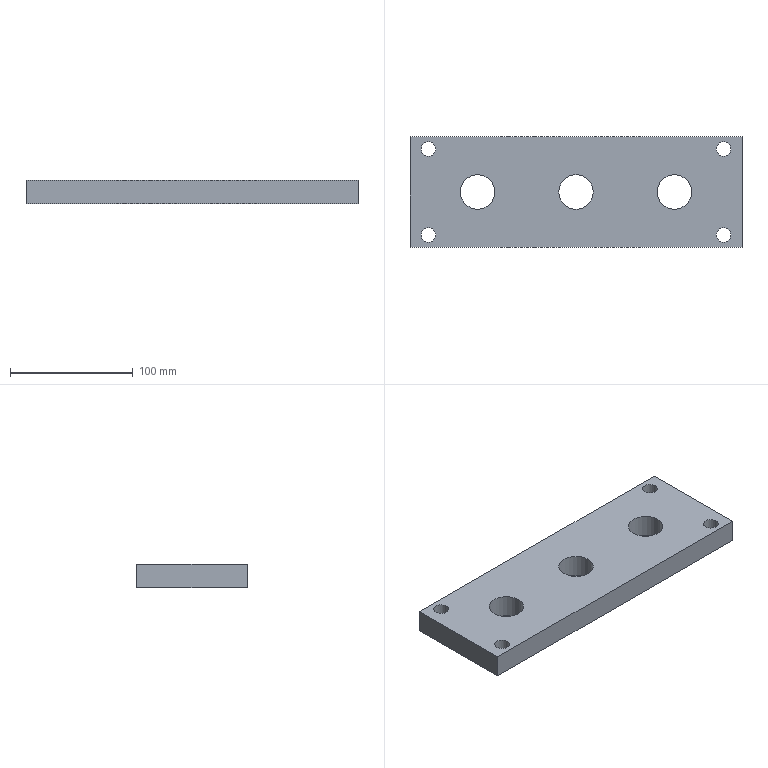Part | NX | features solid 2 | 1 solid | 13 faces | box 270 x 90 x 19 mm | volume 418007 mm3 | cylinder 7 | plane 6 | commonest cylinder face diameters 12 x4 28 x3
STEP:
#1=CARTESIAN_POINT('',(135.,-105.,-30.));
#2=VERTEX_POINT('',#1);
#3=CARTESIAN_POINT('',(-135.,-105.,-30.));
#4=VERTEX_POINT('',#3);
#5=CARTESIAN_POINT('',(165.,-105.,-30.));
#6=DIRECTION('',(-1.,0.,0.));
#7=VECTOR('',#6,1000.);
#8=LINE('',#5,#7);
#9=EDGE_CURVE('',#2,#4,#8,.T.);
#10=ORIENTED_EDGE('',*,*,#9,.T.);
#11=CARTESIAN_POINT('',(-135.,-105.,-49.));
#12=VERTEX_POINT('',#11);
#13=CARTESIAN_POINT('',(-135.,-105.,-30.));
#14=DIRECTION('',(0.,0.,-1.));
#15=VECTOR('',#14,1000.);
#16=LINE('',#13,#15);
#17=EDGE_CURVE('',#4,#12,#16,.T.);
#18=ORIENTED_EDGE('',*,*,#17,.T.);
#19=CARTESIAN_POINT('',(135.,-105.,-49.));
#20=VERTEX_POINT('',#19);
#21=CARTESIAN_POINT('',(-165.,-105.,-49.));
#22=DIRECTION('',(1.,0.,0.));
#23=VECTOR('',#22,1000.);
#24=LINE('',#21,#23);
#25=EDGE_CURVE('',#12,#20,#24,.T.);
#26=ORIENTED_EDGE('',*,*,#25,.T.);
#27=CARTESIAN_POINT('',(135.,-105.,-30.));
#28=DIRECTION('',(0.,0.,-1.));
#29=VECTOR('',#28,1000.);
#30=LINE('',#27,#29);
#31=EDGE_CURVE('',#2,#20,#30,.T.);
#32=ORIENTED_EDGE('',*,*,#31,.F.);
#33=EDGE_LOOP('',(#10,#18,#26,#32));
#34=FACE_BOUND('',#33,.T.);
#35=CARTESIAN_POINT('',(-165.,-105.,-30.));
#36=DIRECTION('',(0.,1.,0.));
#37=DIRECTION('',(0.,0.,1.));
#38=AXIS2_PLACEMENT_3D('',#35,#36,#37);
#39=PLANE('',#38);
#40=ADVANCED_FACE('',(#34),#39,.F.);
#41=CARTESIAN_POINT('',(135.,-15.,-49.));
#42=VERTEX_POINT('',#41);
#43=CARTESIAN_POINT('',(-135.,-15.,-49.));
#44=VERTEX_POINT('',#43);
#45=CARTESIAN_POINT('',(165.,-15.,-49.));
#46=DIRECTION('',(-1.,0.,0.));
#47=VECTOR('',#46,1000.);
#48=LINE('',#45,#47);
#49=EDGE_CURVE('',#42,#44,#48,.T.);
#50=ORIENTED_EDGE('',*,*,#49,.T.);
#51=CARTESIAN_POINT('',(-135.,-15.,-30.));
#52=VERTEX_POINT('',#51);
#53=CARTESIAN_POINT('',(-135.,-15.,-30.));
#54=DIRECTION('',(0.,0.,-1.));
#55=VECTOR('',#54,1000.);
#56=LINE('',#53,#55);
#57=EDGE_CURVE('',#52,#44,#56,.T.);
#58=ORIENTED_EDGE('',*,*,#57,.F.);
#59=CARTESIAN_POINT('',(135.,-15.,-30.));
#60=VERTEX_POINT('',#59);
#61=CARTESIAN_POINT('',(-165.,-15.,-30.));
#62=DIRECTION('',(1.,0.,0.));
#63=VECTOR('',#62,1000.);
#64=LINE('',#61,#63);
#65=EDGE_CURVE('',#52,#60,#64,.T.);
#66=ORIENTED_EDGE('',*,*,#65,.T.);
#67=CARTESIAN_POINT('',(135.,-15.,-30.));
#68=DIRECTION('',(0.,0.,-1.));
#69=VECTOR('',#68,1000.);
#70=LINE('',#67,#69);
#71=EDGE_CURVE('',#60,#42,#70,.T.);
#72=ORIENTED_EDGE('',*,*,#71,.T.);
#73=EDGE_LOOP('',(#50,#58,#66,#72));
#74=FACE_BOUND('',#73,.T.);
#75=CARTESIAN_POINT('',(165.,-15.,-30.));
#76=DIRECTION('',(0.,-1.,0.));
#77=DIRECTION('',(1.,0.,0.));
#78=AXIS2_PLACEMENT_3D('',#75,#76,#77);
#79=PLANE('',#78);
#80=ADVANCED_FACE('',(#74),#79,.F.);
#81=CARTESIAN_POINT('',(-114.,-25.,-30.));
#82=VERTEX_POINT('',#81);
#83=CARTESIAN_POINT('',(-120.,-25.,-30.));
#84=DIRECTION('',(0.,0.,1.));
#85=DIRECTION('',(1.,0.,0.));
#86=AXIS2_PLACEMENT_3D('',#83,#84,#85);
#87=CIRCLE('',#86,6.);
#88=EDGE_CURVE('',#82,#82,#87,.T.);
#89=ORIENTED_EDGE('',*,*,#88,.T.);
#90=EDGE_LOOP('',(#89));
#91=FACE_BOUND('',#90,.T.);
#92=CARTESIAN_POINT('',(-114.,-25.,-49.));
#93=VERTEX_POINT('',#92);
#94=CARTESIAN_POINT('',(-120.,-25.,-49.));
#95=DIRECTION('',(0.,0.,1.));
#96=DIRECTION('',(1.,0.,0.));
#97=AXIS2_PLACEMENT_3D('',#94,#95,#96);
#98=CIRCLE('',#97,6.);
#99=EDGE_CURVE('',#93,#93,#98,.T.);
#100=ORIENTED_EDGE('',*,*,#99,.F.);
#101=EDGE_LOOP('',(#100));
#102=FACE_BOUND('',#101,.T.);
#103=CARTESIAN_POINT('',(-120.,-25.,-30.));
#104=DIRECTION('',(0.,0.,-1.));
#105=DIRECTION('',(-1.,0.,0.));
#106=AXIS2_PLACEMENT_3D('',#103,#104,#105);
#107=CYLINDRICAL_SURFACE('',#106,6.);
#108=ADVANCED_FACE('',(#91,#102),#107,.F.);
#109=CARTESIAN_POINT('',(-114.,-95.,-30.));
#110=VERTEX_POINT('',#109);
#111=CARTESIAN_POINT('',(-120.,-95.,-30.));
#112=DIRECTION('',(0.,0.,-1.));
#113=DIRECTION('',(1.,0.,0.));
#114=AXIS2_PLACEMENT_3D('',#111,#112,#113);
#115=CIRCLE('',#114,6.);
#116=EDGE_CURVE('',#110,#110,#115,.T.);
#117=ORIENTED_EDGE('',*,*,#116,.F.);
#118=EDGE_LOOP('',(#117));
#119=FACE_BOUND('',#118,.T.);
#120=CARTESIAN_POINT('',(-114.,-95.,-49.));
#121=VERTEX_POINT('',#120);
#122=CARTESIAN_POINT('',(-120.,-95.,-49.));
#123=DIRECTION('',(0.,0.,-1.));
#124=DIRECTION('',(1.,0.,0.));
#125=AXIS2_PLACEMENT_3D('',#122,#123,#124);
#126=CIRCLE('',#125,6.);
#127=EDGE_CURVE('',#121,#121,#126,.T.);
#128=ORIENTED_EDGE('',*,*,#127,.T.);
#129=EDGE_LOOP('',(#128));
#130=FACE_BOUND('',#129,.T.);
#131=CARTESIAN_POINT('',(-120.,-95.,-30.));
#132=DIRECTION('',(0.,0.,-1.));
#133=DIRECTION('',(-1.,0.,0.));
#134=AXIS2_PLACEMENT_3D('',#131,#132,#133);
#135=CYLINDRICAL_SURFACE('',#134,6.);
#136=ADVANCED_FACE('',(#119,#130),#135,.F.);
#137=CARTESIAN_POINT('',(114.,-25.,-30.));
#138=VERTEX_POINT('',#137);
#139=CARTESIAN_POINT('',(120.,-25.,-30.));
#140=DIRECTION('',(0.,0.,-1.));
#141=DIRECTION('',(-1.,0.,0.));
#142=AXIS2_PLACEMENT_3D('',#139,#140,#141);
#143=CIRCLE('',#142,6.);
#144=EDGE_CURVE('',#138,#138,#143,.T.);
#145=ORIENTED_EDGE('',*,*,#144,.F.);
#146=EDGE_LOOP('',(#145));
#147=FACE_BOUND('',#146,.T.);
#148=CARTESIAN_POINT('',(114.,-25.,-49.));
#149=VERTEX_POINT('',#148);
#150=CARTESIAN_POINT('',(120.,-25.,-49.));
#151=DIRECTION('',(0.,0.,-1.));
#152=DIRECTION('',(-1.,0.,0.));
#153=AXIS2_PLACEMENT_3D('',#150,#151,#152);
#154=CIRCLE('',#153,6.);
#155=EDGE_CURVE('',#149,#149,#154,.T.);
#156=ORIENTED_EDGE('',*,*,#155,.T.);
#157=EDGE_LOOP('',(#156));
#158=FACE_BOUND('',#157,.T.);
#159=CARTESIAN_POINT('',(120.,-25.,-30.));
#160=DIRECTION('',(0.,0.,-1.));
#161=DIRECTION('',(-1.,0.,0.));
#162=AXIS2_PLACEMENT_3D('',#159,#160,#161);
#163=CYLINDRICAL_SURFACE('',#162,6.);
#164=ADVANCED_FACE('',(#147,#158),#163,.F.);
#165=CARTESIAN_POINT('',(114.,-95.,-30.));
#166=VERTEX_POINT('',#165);
#167=CARTESIAN_POINT('',(120.,-95.,-30.));
#168=DIRECTION('',(0.,0.,1.));
#169=DIRECTION('',(-1.,0.,0.));
#170=AXIS2_PLACEMENT_3D('',#167,#168,#169);
#171=CIRCLE('',#170,6.);
#172=EDGE_CURVE('',#166,#166,#171,.T.);
#173=ORIENTED_EDGE('',*,*,#172,.T.);
#174=EDGE_LOOP('',(#173));
#175=FACE_BOUND('',#174,.T.);
#176=CARTESIAN_POINT('',(114.,-95.,-49.));
#177=VERTEX_POINT('',#176);
#178=CARTESIAN_POINT('',(120.,-95.,-49.));
#179=DIRECTION('',(0.,0.,1.));
#180=DIRECTION('',(-1.,0.,0.));
#181=AXIS2_PLACEMENT_3D('',#178,#179,#180);
#182=CIRCLE('',#181,6.);
#183=EDGE_CURVE('',#177,#177,#182,.T.);
#184=ORIENTED_EDGE('',*,*,#183,.F.);
#185=EDGE_LOOP('',(#184));
#186=FACE_BOUND('',#185,.T.);
#187=CARTESIAN_POINT('',(120.,-95.,-30.));
#188=DIRECTION('',(0.,0.,-1.));
#189=DIRECTION('',(-1.,0.,0.));
#190=AXIS2_PLACEMENT_3D('',#187,#188,#189);
#191=CYLINDRICAL_SURFACE('',#190,6.);
#192=ADVANCED_FACE('',(#175,#186),#191,.F.);
#193=CARTESIAN_POINT('',(66.,-60.,-30.));
#194=VERTEX_POINT('',#193);
#195=CARTESIAN_POINT('',(80.,-60.,-30.));
#196=DIRECTION('',(0.,0.,-1.));
#197=DIRECTION('',(-1.,0.,0.));
#198=AXIS2_PLACEMENT_3D('',#195,#196,#197);
#199=CIRCLE('',#198,14.);
#200=EDGE_CURVE('',#194,#194,#199,.T.);
#201=ORIENTED_EDGE('',*,*,#200,.F.);
#202=EDGE_LOOP('',(#201));
#203=FACE_BOUND('',#202,.T.);
#204=CARTESIAN_POINT('',(66.,-60.,-49.));
#205=VERTEX_POINT('',#204);
#206=CARTESIAN_POINT('',(80.,-60.,-49.));
#207=DIRECTION('',(0.,0.,-1.));
#208=DIRECTION('',(-1.,0.,0.));
#209=AXIS2_PLACEMENT_3D('',#206,#207,#208);
#210=CIRCLE('',#209,14.);
#211=EDGE_CURVE('',#205,#205,#210,.T.);
#212=ORIENTED_EDGE('',*,*,#211,.T.);
#213=EDGE_LOOP('',(#212));
#214=FACE_BOUND('',#213,.T.);
#215=CARTESIAN_POINT('',(80.,-60.,-30.));
#216=DIRECTION('',(0.,0.,-1.));
#217=DIRECTION('',(-1.,0.,0.));
#218=AXIS2_PLACEMENT_3D('',#215,#216,#217);
#219=CYLINDRICAL_SURFACE('',#218,14.);
#220=ADVANCED_FACE('',(#203,#214),#219,.F.);
#221=CARTESIAN_POINT('',(14.,-60.,-30.));
#222=VERTEX_POINT('',#221);
#223=CARTESIAN_POINT('',(0.,-60.,-30.));
#224=DIRECTION('',(0.,0.,1.));
#225=DIRECTION('',(1.,0.,0.));
#226=AXIS2_PLACEMENT_3D('',#223,#224,#225);
#227=CIRCLE('',#226,14.);
#228=EDGE_CURVE('',#222,#222,#227,.T.);
#229=ORIENTED_EDGE('',*,*,#228,.T.);
#230=EDGE_LOOP('',(#229));
#231=FACE_BOUND('',#230,.T.);
#232=CARTESIAN_POINT('',(14.,-60.,-49.));
#233=VERTEX_POINT('',#232);
#234=CARTESIAN_POINT('',(0.,-60.,-49.));
#235=DIRECTION('',(0.,0.,1.));
#236=DIRECTION('',(1.,0.,0.));
#237=AXIS2_PLACEMENT_3D('',#234,#235,#236);
#238=CIRCLE('',#237,14.);
#239=EDGE_CURVE('',#233,#233,#238,.T.);
#240=ORIENTED_EDGE('',*,*,#239,.F.);
#241=EDGE_LOOP('',(#240));
#242=FACE_BOUND('',#241,.T.);
#243=CARTESIAN_POINT('',(0.,-60.,-30.));
#244=DIRECTION('',(0.,0.,-1.));
#245=DIRECTION('',(-1.,0.,0.));
#246=AXIS2_PLACEMENT_3D('',#243,#244,#245);
#247=CYLINDRICAL_SURFACE('',#246,14.);
#248=ADVANCED_FACE('',(#231,#242),#247,.F.);
#249=CARTESIAN_POINT('',(-66.,-60.,-30.));
#250=VERTEX_POINT('',#249);
#251=CARTESIAN_POINT('',(-80.,-60.,-30.));
#252=DIRECTION('',(0.,0.,1.));
#253=DIRECTION('',(1.,0.,0.));
#254=AXIS2_PLACEMENT_3D('',#251,#252,#253);
#255=CIRCLE('',#254,14.);
#256=EDGE_CURVE('',#250,#250,#255,.T.);
#257=ORIENTED_EDGE('',*,*,#256,.T.);
#258=EDGE_LOOP('',(#257));
#259=FACE_BOUND('',#258,.T.);
#260=CARTESIAN_POINT('',(-66.,-60.,-49.));
#261=VERTEX_POINT('',#260);
#262=CARTESIAN_POINT('',(-80.,-60.,-49.));
#263=DIRECTION('',(0.,0.,1.));
#264=DIRECTION('',(1.,0.,0.));
#265=AXIS2_PLACEMENT_3D('',#262,#263,#264);
#266=CIRCLE('',#265,14.);
#267=EDGE_CURVE('',#261,#261,#266,.T.);
#268=ORIENTED_EDGE('',*,*,#267,.F.);
#269=EDGE_LOOP('',(#268));
#270=FACE_BOUND('',#269,.T.);
#271=CARTESIAN_POINT('',(-80.,-60.,-30.));
#272=DIRECTION('',(0.,0.,-1.));
#273=DIRECTION('',(-1.,0.,0.));
#274=AXIS2_PLACEMENT_3D('',#271,#272,#273);
#275=CYLINDRICAL_SURFACE('',#274,14.);
#276=ADVANCED_FACE('',(#259,#270),#275,.F.);
#277=CARTESIAN_POINT('',(-135.,-15.,-30.));
#278=DIRECTION('',(0.,-1.,0.));
#279=VECTOR('',#278,1000.);
#280=LINE('',#277,#279);
#281=EDGE_CURVE('',#52,#4,#280,.T.);
#282=ORIENTED_EDGE('',*,*,#281,.T.);
#283=ORIENTED_EDGE('',*,*,#9,.F.);
#284=CARTESIAN_POINT('',(135.,-105.,-30.));
#285=DIRECTION('',(0.,1.,0.));
#286=VECTOR('',#285,1000.);
#287=LINE('',#284,#286);
#288=EDGE_CURVE('',#2,#60,#287,.T.);
#289=ORIENTED_EDGE('',*,*,#288,.T.);
#290=ORIENTED_EDGE('',*,*,#65,.F.);
#291=EDGE_LOOP('',(#282,#283,#289,#290));
#292=FACE_BOUND('',#291,.T.);
#293=ORIENTED_EDGE('',*,*,#228,.F.);
#294=EDGE_LOOP('',(#293));
#295=FACE_BOUND('',#294,.T.);
#296=ORIENTED_EDGE('',*,*,#200,.T.);
#297=EDGE_LOOP('',(#296));
#298=FACE_BOUND('',#297,.T.);
#299=ORIENTED_EDGE('',*,*,#172,.F.);
#300=EDGE_LOOP('',(#299));
#301=FACE_BOUND('',#300,.T.);
#302=ORIENTED_EDGE('',*,*,#144,.T.);
#303=EDGE_LOOP('',(#302));
#304=FACE_BOUND('',#303,.T.);
#305=ORIENTED_EDGE('',*,*,#116,.T.);
#306=EDGE_LOOP('',(#305));
#307=FACE_BOUND('',#306,.T.);
#308=ORIENTED_EDGE('',*,*,#88,.F.);
#309=EDGE_LOOP('',(#308));
#310=FACE_BOUND('',#309,.T.);
#311=ORIENTED_EDGE('',*,*,#256,.F.);
#312=EDGE_LOOP('',(#311));
#313=FACE_BOUND('',#312,.T.);
#314=CARTESIAN_POINT('',(165.,-15.,-30.));
#315=DIRECTION('',(0.,0.,1.));
#316=DIRECTION('',(1.,0.,0.));
#317=AXIS2_PLACEMENT_3D('',#314,#315,#316);
#318=PLANE('',#317);
#319=ADVANCED_FACE('',(#292,#295,#298,#301,#304,#307,#310,#313),#318,.T.);
#320=ORIENTED_EDGE('',*,*,#239,.T.);
#321=EDGE_LOOP('',(#320));
#322=FACE_BOUND('',#321,.T.);
#323=ORIENTED_EDGE('',*,*,#211,.F.);
#324=EDGE_LOOP('',(#323));
#325=FACE_BOUND('',#324,.T.);
#326=ORIENTED_EDGE('',*,*,#183,.T.);
#327=EDGE_LOOP('',(#326));
#328=FACE_BOUND('',#327,.T.);
#329=ORIENTED_EDGE('',*,*,#25,.F.);
#330=CARTESIAN_POINT('',(-135.,-15.,-49.));
#331=DIRECTION('',(0.,-1.,0.));
#332=VECTOR('',#331,1000.);
#333=LINE('',#330,#332);
#334=EDGE_CURVE('',#44,#12,#333,.T.);
#335=ORIENTED_EDGE('',*,*,#334,.F.);
#336=ORIENTED_EDGE('',*,*,#49,.F.);
#337=CARTESIAN_POINT('',(135.,-105.,-49.));
#338=DIRECTION('',(0.,1.,0.));
#339=VECTOR('',#338,1000.);
#340=LINE('',#337,#339);
#341=EDGE_CURVE('',#20,#42,#340,.T.);
#342=ORIENTED_EDGE('',*,*,#341,.F.);
#343=EDGE_LOOP('',(#329,#335,#336,#342));
#344=FACE_BOUND('',#343,.T.);
#345=ORIENTED_EDGE('',*,*,#155,.F.);
#346=EDGE_LOOP('',(#345));
#347=FACE_BOUND('',#346,.T.);
#348=ORIENTED_EDGE('',*,*,#127,.F.);
#349=EDGE_LOOP('',(#348));
#350=FACE_BOUND('',#349,.T.);
#351=ORIENTED_EDGE('',*,*,#99,.T.);
#352=EDGE_LOOP('',(#351));
#353=FACE_BOUND('',#352,.T.);
#354=ORIENTED_EDGE('',*,*,#267,.T.);
#355=EDGE_LOOP('',(#354));
#356=FACE_BOUND('',#355,.T.);
#357=CARTESIAN_POINT('',(165.,-15.,-49.));
#358=DIRECTION('',(0.,0.,1.));
#359=DIRECTION('',(1.,0.,0.));
#360=AXIS2_PLACEMENT_3D('',#357,#358,#359);
#361=PLANE('',#360);
#362=ADVANCED_FACE('',(#322,#325,#328,#344,#347,#350,#353,#356),#361,.F.);
#363=ORIENTED_EDGE('',*,*,#341,.T.);
#364=ORIENTED_EDGE('',*,*,#71,.F.);
#365=ORIENTED_EDGE('',*,*,#288,.F.);
#366=ORIENTED_EDGE('',*,*,#31,.T.);
#367=EDGE_LOOP('',(#363,#364,#365,#366));
#368=FACE_BOUND('',#367,.T.);
#369=CARTESIAN_POINT('',(135.,-105.,-30.));
#370=DIRECTION('',(-1.,0.,0.));
#371=DIRECTION('',(0.,-1.,0.));
#372=AXIS2_PLACEMENT_3D('',#369,#370,#371);
#373=PLANE('',#372);
#374=ADVANCED_FACE('',(#368),#373,.F.);
#375=ORIENTED_EDGE('',*,*,#334,.T.);
#376=ORIENTED_EDGE('',*,*,#17,.F.);
#377=ORIENTED_EDGE('',*,*,#281,.F.);
#378=ORIENTED_EDGE('',*,*,#57,.T.);
#379=EDGE_LOOP('',(#375,#376,#377,#378));
#380=FACE_BOUND('',#379,.T.);
#381=CARTESIAN_POINT('',(-135.,-15.,-30.));
#382=DIRECTION('',(1.,0.,0.));
#383=DIRECTION('',(0.,1.,0.));
#384=AXIS2_PLACEMENT_3D('',#381,#382,#383);
#385=PLANE('',#384);
#386=ADVANCED_FACE('',(#380),#385,.F.);
#387=CLOSED_SHELL('',(#40,#80,#108,#136,#164,#192,#220,#248,#276,#319,#362,#374,#386));
#388=MANIFOLD_SOLID_BREP('',#387);
#389=(LENGTH_UNIT()NAMED_UNIT(*)SI_UNIT(.MILLI.,.METRE.));
#390=UNCERTAINTY_MEASURE_WITH_UNIT(LENGTH_MEASURE(0.00001),#389,'','');
#391=(NAMED_UNIT(*)PLANE_ANGLE_UNIT()SI_UNIT($,.RADIAN.));
#392=(NAMED_UNIT(*)SI_UNIT($,.STERADIAN.)SOLID_ANGLE_UNIT());
#393=(GEOMETRIC_REPRESENTATION_CONTEXT(3)GLOBAL_UNCERTAINTY_ASSIGNED_CONTEXT((#390))GLOBAL_UNIT_ASSIGNED_CONTEXT((#389,#391,#392))REPRESENTATION_CONTEXT('',''));
#394=ADVANCED_BREP_SHAPE_REPRESENTATION('',(#388),#393);